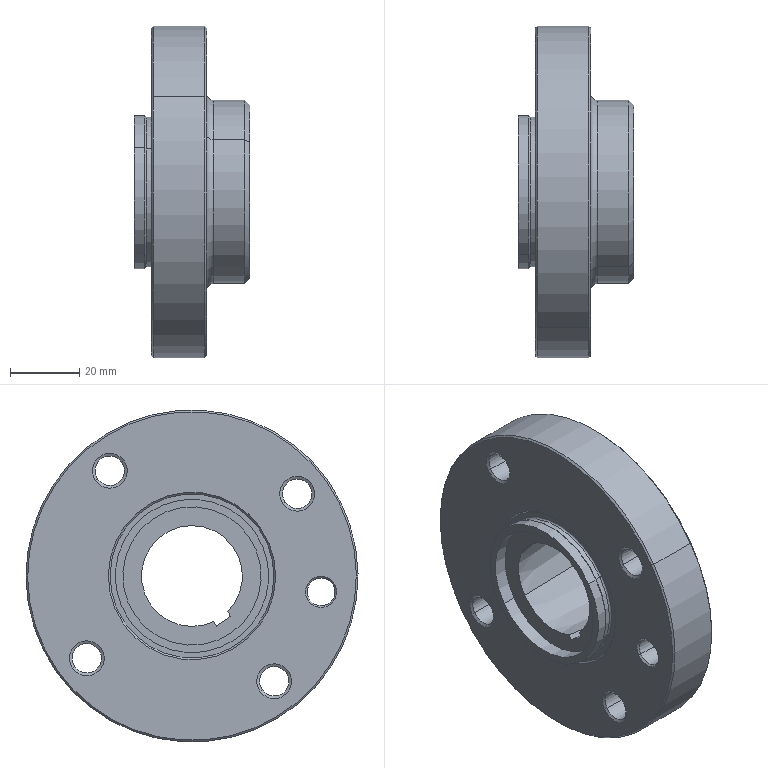Part | SolidWorks | features BaseBody 1 | 1 solid | 66 faces | box 33.5 x 96 x 96 mm | volume 117119 mm3 | cone 33 | cylinder 20 | plane 9 | torus 4 | commonest cylinder face diameters 8.5 x8 8 x2 40 x2 43.4 x2 44.4 x2 53 x2